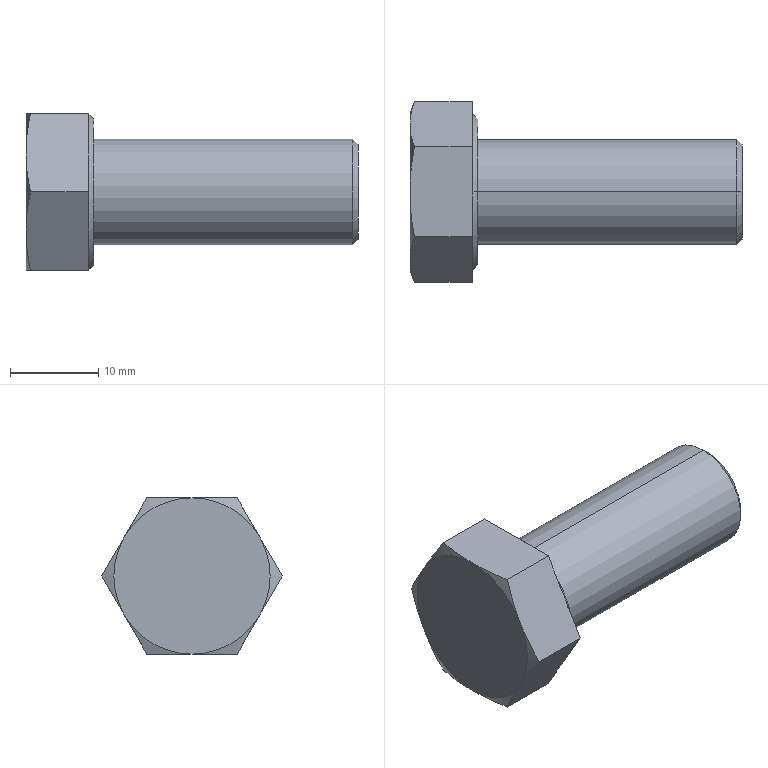Part | SolidWorks | features RevCut 3, Boss 1, Chamfer 1, Extrusion 1, Fillet 1, LPattern 1 | 1 solid | 27 faces | box 37.68 x 20.473 x 17.73 mm | volume 5450 mm3 | plane 15 | cone 10 | cylinder 2 | commonest cylinder face diameters 12 x2
STEP:
#1=CARTESIAN_POINT('',(37.68,0.,-5.4));
#2=VERTEX_POINT('',#1);
#3=CARTESIAN_POINT('',(37.68,0.,5.4));
#4=VERTEX_POINT('',#3);
#5=CARTESIAN_POINT('',(37.68,0.,0.));
#6=DIRECTION('',(1.,0.,0.));
#7=DIRECTION('',(0.,0.,-1.));
#8=AXIS2_PLACEMENT_3D('',#5,#6,#7);
#9=CIRCLE('',#8,5.4);
#10=EDGE_CURVE('',#2,#4,#9,.T.);
#11=ORIENTED_EDGE('',*,*,#10,.F.);
#12=CARTESIAN_POINT('',(37.08,0.,-6.));
#13=VERTEX_POINT('',#12);
#14=CARTESIAN_POINT('',(37.68,0.,-5.4));
#15=DIRECTION('',(-0.7071,0.,-0.7071));
#16=VECTOR('',#15,1000.);
#17=LINE('',#14,#16);
#18=EDGE_CURVE('',#2,#13,#17,.T.);
#19=ORIENTED_EDGE('',*,*,#18,.T.);
#20=CARTESIAN_POINT('',(37.08,0.,6.));
#21=VERTEX_POINT('',#20);
#22=CARTESIAN_POINT('',(37.08,0.,0.));
#23=DIRECTION('',(-1.,0.,0.));
#24=DIRECTION('',(0.,0.,-1.));
#25=AXIS2_PLACEMENT_3D('',#22,#23,#24);
#26=CIRCLE('',#25,6.);
#27=EDGE_CURVE('',#21,#13,#26,.T.);
#28=ORIENTED_EDGE('',*,*,#27,.F.);
#29=CARTESIAN_POINT('',(37.68,0.,5.4));
#30=DIRECTION('',(-0.7071,0.,0.7071));
#31=VECTOR('',#30,1000.);
#32=LINE('',#29,#31);
#33=EDGE_CURVE('',#4,#21,#32,.T.);
#34=ORIENTED_EDGE('',*,*,#33,.F.);
#35=EDGE_LOOP('',(#11,#19,#28,#34));
#36=FACE_OUTER_BOUND('',#35,.T.);
#37=CARTESIAN_POINT('',(37.68,0.,0.));
#38=DIRECTION('',(-1.,0.,0.));
#39=DIRECTION('',(0.,0.,1.));
#40=AXIS2_PLACEMENT_3D('',#37,#38,#39);
#41=CONICAL_SURFACE('',#40,5.4,0.7854);
#42=ADVANCED_FACE('',(#36),#41,.T.);
#43=ORIENTED_EDGE('',*,*,#27,.T.);
#44=CARTESIAN_POINT('',(7.68,0.,-6.));
#45=VERTEX_POINT('',#44);
#46=CARTESIAN_POINT('',(37.68,0.,-6.));
#47=DIRECTION('',(-1.,0.,0.));
#48=VECTOR('',#47,1000.);
#49=LINE('',#46,#48);
#50=EDGE_CURVE('',#13,#45,#49,.T.);
#51=ORIENTED_EDGE('',*,*,#50,.T.);
#52=CARTESIAN_POINT('',(7.68,0.,6.));
#53=VERTEX_POINT('',#52);
#54=CARTESIAN_POINT('',(7.68,0.,0.));
#55=DIRECTION('',(1.,0.,0.));
#56=DIRECTION('',(0.,0.,-1.));
#57=AXIS2_PLACEMENT_3D('',#54,#55,#56);
#58=CIRCLE('',#57,6.);
#59=EDGE_CURVE('',#45,#53,#58,.T.);
#60=ORIENTED_EDGE('',*,*,#59,.T.);
#61=CARTESIAN_POINT('',(37.68,0.,6.));
#62=DIRECTION('',(-1.,0.,0.));
#63=VECTOR('',#62,1000.);
#64=LINE('',#61,#63);
#65=EDGE_CURVE('',#21,#53,#64,.T.);
#66=ORIENTED_EDGE('',*,*,#65,.F.);
#67=EDGE_LOOP('',(#43,#51,#60,#66));
#68=FACE_OUTER_BOUND('',#67,.T.);
#69=CARTESIAN_POINT('',(37.68,0.,0.));
#70=DIRECTION('',(-1.,0.,0.));
#71=DIRECTION('',(0.,0.,1.));
#72=AXIS2_PLACEMENT_3D('',#69,#70,#71);
#73=CYLINDRICAL_SURFACE('',#72,6.);
#74=ADVANCED_FACE('',(#68),#73,.T.);
#75=CARTESIAN_POINT('',(7.68,0.,8.315));
#76=VERTEX_POINT('',#75);
#77=CARTESIAN_POINT('',(7.68,0.,-8.315));
#78=VERTEX_POINT('',#77);
#79=CARTESIAN_POINT('',(7.68,0.,0.));
#80=DIRECTION('',(-1.,0.,0.));
#81=DIRECTION('',(0.,0.,1.));
#82=AXIS2_PLACEMENT_3D('',#79,#80,#81);
#83=CIRCLE('',#82,8.315);
#84=EDGE_CURVE('',#76,#78,#83,.T.);
#85=ORIENTED_EDGE('',*,*,#84,.T.);
#86=CARTESIAN_POINT('',(7.13,0.,-8.865));
#87=VERTEX_POINT('',#86);
#88=CARTESIAN_POINT('',(7.08,0.,-8.915));
#89=DIRECTION('',(-0.7071,0.,-0.7071));
#90=VECTOR('',#89,1000.);
#91=LINE('',#88,#90);
#92=EDGE_CURVE('',#78,#87,#91,.T.);
#93=ORIENTED_EDGE('',*,*,#92,.T.);
#94=CARTESIAN_POINT('',(7.08,0.9429,-8.865));
#95=VERTEX_POINT('',#94);
#96=CARTESIAN_POINT('',(7.13,0.,-8.865));
#97=CARTESIAN_POINT('',(7.13,0.3145,-8.865));
#98=CARTESIAN_POINT('',(7.113,0.6288,-8.865));
#99=CARTESIAN_POINT('',(7.08,0.9429,-8.865));
#100=B_SPLINE_CURVE_WITH_KNOTS('',3,(#96,#97,#98,#99),.UNSPECIFIED.,.F.,.F.,(4,4),(0.004972,0.005912),.UNSPECIFIED.);
#101=EDGE_CURVE('',#87,#95,#100,.T.);
#102=ORIENTED_EDGE('',*,*,#101,.T.);
#103=CARTESIAN_POINT('',(7.08,7.206,-5.249));
#104=VERTEX_POINT('',#103);
#105=CARTESIAN_POINT('',(7.08,0.,0.));
#106=DIRECTION('',(-1.,0.,0.));
#107=DIRECTION('',(0.,0.,1.));
#108=AXIS2_PLACEMENT_3D('',#105,#106,#107);
#109=CIRCLE('',#108,8.915);
#110=EDGE_CURVE('',#104,#95,#109,.T.);
#111=ORIENTED_EDGE('',*,*,#110,.F.);
#112=CARTESIAN_POINT('',(7.08,8.149,-3.616));
#113=VERTEX_POINT('',#112);
#114=CARTESIAN_POINT('',(7.08,7.206,-5.249));
#115=CARTESIAN_POINT('',(7.146,7.52,-4.705));
#116=CARTESIAN_POINT('',(7.146,7.834,-4.16));
#117=CARTESIAN_POINT('',(7.08,8.149,-3.616));
#118=B_SPLINE_CURVE_WITH_KNOTS('',3,(#114,#115,#116,#117),.UNSPECIFIED.,.F.,.F.,(4,4),(0.000001889,0.001888),.UNSPECIFIED.);
#119=EDGE_CURVE('',#104,#113,#118,.T.);
#120=ORIENTED_EDGE('',*,*,#119,.T.);
#121=CARTESIAN_POINT('',(7.08,8.149,3.616));
#122=VERTEX_POINT('',#121);
#123=CARTESIAN_POINT('',(7.08,0.,0.));
#124=DIRECTION('',(-1.,0.,0.));
#125=DIRECTION('',(0.,0.,1.));
#126=AXIS2_PLACEMENT_3D('',#123,#124,#125);
#127=CIRCLE('',#126,8.915);
#128=EDGE_CURVE('',#122,#113,#127,.T.);
#129=ORIENTED_EDGE('',*,*,#128,.F.);
#130=CARTESIAN_POINT('',(7.08,7.206,5.249));
#131=VERTEX_POINT('',#130);
#132=CARTESIAN_POINT('',(7.08,8.149,3.616));
#133=CARTESIAN_POINT('',(7.146,7.834,4.16));
#134=CARTESIAN_POINT('',(7.146,7.52,4.705));
#135=CARTESIAN_POINT('',(7.08,7.206,5.249));
#136=B_SPLINE_CURVE_WITH_KNOTS('',3,(#132,#133,#134,#135),.UNSPECIFIED.,.F.,.F.,(4,4),(0.000001889,0.001888),.UNSPECIFIED.);
#137=EDGE_CURVE('',#122,#131,#136,.T.);
#138=ORIENTED_EDGE('',*,*,#137,.T.);
#139=CARTESIAN_POINT('',(7.08,0.9429,8.865));
#140=VERTEX_POINT('',#139);
#141=CARTESIAN_POINT('',(7.08,0.,0.));
#142=DIRECTION('',(-1.,0.,0.));
#143=DIRECTION('',(0.,0.,1.));
#144=AXIS2_PLACEMENT_3D('',#141,#142,#143);
#145=CIRCLE('',#144,8.915);
#146=EDGE_CURVE('',#140,#131,#145,.T.);
#147=ORIENTED_EDGE('',*,*,#146,.F.);
#148=CARTESIAN_POINT('',(7.13,0.,8.865));
#149=VERTEX_POINT('',#148);
#150=CARTESIAN_POINT('',(7.08,0.9429,8.865));
#151=CARTESIAN_POINT('',(7.113,0.6288,8.865));
#152=CARTESIAN_POINT('',(7.13,0.3145,8.865));
#153=CARTESIAN_POINT('',(7.13,0.,8.865));
#154=B_SPLINE_CURVE_WITH_KNOTS('',3,(#150,#151,#152,#153),.UNSPECIFIED.,.F.,.F.,(4,4),(0.004457,0.005396),.UNSPECIFIED.);
#155=EDGE_CURVE('',#140,#149,#154,.T.);
#156=ORIENTED_EDGE('',*,*,#155,.T.);
#157=CARTESIAN_POINT('',(7.08,0.,8.915));
#158=DIRECTION('',(-0.7071,0.,0.7071));
#159=VECTOR('',#158,1000.);
#160=LINE('',#157,#159);
#161=EDGE_CURVE('',#76,#149,#160,.T.);
#162=ORIENTED_EDGE('',*,*,#161,.F.);
#163=EDGE_LOOP('',(#85,#93,#102,#111,#120,#129,#138,#147,#156,#162));
#164=FACE_OUTER_BOUND('',#163,.T.);
#165=CARTESIAN_POINT('',(7.08,0.,0.));
#166=DIRECTION('',(-1.,0.,0.));
#167=DIRECTION('',(0.,0.,1.));
#168=AXIS2_PLACEMENT_3D('',#165,#166,#167);
#169=CONICAL_SURFACE('',#168,8.915,0.7854);
#170=ADVANCED_FACE('',(#164),#169,.T.);
#171=ORIENTED_EDGE('',*,*,#84,.F.);
#172=CARTESIAN_POINT('',(7.68,0.,0.));
#173=DIRECTION('',(-1.,0.,0.));
#174=DIRECTION('',(0.,0.,1.));
#175=AXIS2_PLACEMENT_3D('',#172,#173,#174);
#176=CIRCLE('',#175,8.315);
#177=EDGE_CURVE('',#78,#76,#176,.T.);
#178=ORIENTED_EDGE('',*,*,#177,.F.);
#179=EDGE_LOOP('',(#171,#178));
#180=FACE_OUTER_BOUND('',#179,.T.);
#181=CARTESIAN_POINT('',(7.68,0.,0.));
#182=DIRECTION('',(1.,0.,0.));
#183=DIRECTION('',(0.,0.,-1.));
#184=AXIS2_PLACEMENT_3D('',#181,#182,#183);
#185=CIRCLE('',#184,6.);
#186=EDGE_CURVE('',#53,#45,#185,.T.);
#187=ORIENTED_EDGE('',*,*,#186,.F.);
#188=ORIENTED_EDGE('',*,*,#59,.F.);
#189=EDGE_LOOP('',(#187,#188));
#190=FACE_BOUND('',#189,.T.);
#191=CARTESIAN_POINT('',(7.68,-5.118,-8.865));
#192=DIRECTION('',(1.,0.,0.));
#193=DIRECTION('',(0.,0.,-1.));
#194=AXIS2_PLACEMENT_3D('',#191,#192,#193);
#195=PLANE('',#194);
#196=ADVANCED_FACE('',(#180,#190),#195,.T.);
#197=CARTESIAN_POINT('',(0.4992,-5.118,-8.865));
#198=VERTEX_POINT('',#197);
#199=CARTESIAN_POINT('',(0.,-7.677,-4.432));
#200=VERTEX_POINT('',#199);
#201=CARTESIAN_POINT('',(0.4992,-5.118,-8.865));
#202=CARTESIAN_POINT('',(0.3439,-5.545,-8.126));
#203=CARTESIAN_POINT('',(0.2179,-5.971,-7.388));
#204=CARTESIAN_POINT('',(0.04564,-6.824,-5.91));
#205=CARTESIAN_POINT('',(0.,-7.251,-5.171));
#206=CARTESIAN_POINT('',(0.,-7.677,-4.432));
#207=B_SPLINE_CURVE_WITH_KNOTS('',3,(#201,#202,#203,#204,#205,#206),.UNSPECIFIED.,.F.,.F.,(4,2,4),(0.000000231,0.002559,0.005118),.UNSPECIFIED.);
#208=EDGE_CURVE('',#198,#200,#207,.T.);
#209=ORIENTED_EDGE('',*,*,#208,.F.);
#210=CARTESIAN_POINT('',(7.08,-5.118,-8.865));
#211=VERTEX_POINT('',#210);
#212=CARTESIAN_POINT('',(7.68,-5.118,-8.865));
#213=DIRECTION('',(-1.,0.,0.));
#214=VECTOR('',#213,1000.);
#215=LINE('',#212,#214);
#216=EDGE_CURVE('',#211,#198,#215,.T.);
#217=ORIENTED_EDGE('',*,*,#216,.F.);
#218=CARTESIAN_POINT('',(7.08,-7.206,-5.249));
#219=VERTEX_POINT('',#218);
#220=CARTESIAN_POINT('',(7.08,-10.236,0.));
#221=DIRECTION('',(0.,0.5,-0.866));
#222=VECTOR('',#221,1000.);
#223=LINE('',#220,#222);
#224=EDGE_CURVE('',#219,#211,#223,.T.);
#225=ORIENTED_EDGE('',*,*,#224,.F.);
#226=CARTESIAN_POINT('',(7.08,-8.149,-3.616));
#227=VERTEX_POINT('',#226);
#228=CARTESIAN_POINT('',(7.08,-8.149,-3.616));
#229=CARTESIAN_POINT('',(7.146,-7.834,-4.16));
#230=CARTESIAN_POINT('',(7.146,-7.52,-4.705));
#231=CARTESIAN_POINT('',(7.08,-7.206,-5.249));
#232=B_SPLINE_CURVE_WITH_KNOTS('',3,(#228,#229,#230,#231),.UNSPECIFIED.,.F.,.F.,(4,4),(0.000001889,0.001888),.UNSPECIFIED.);
#233=EDGE_CURVE('',#227,#219,#232,.T.);
#234=ORIENTED_EDGE('',*,*,#233,.F.);
#235=CARTESIAN_POINT('',(7.08,-10.236,0.));
#236=VERTEX_POINT('',#235);
#237=CARTESIAN_POINT('',(7.08,-10.236,0.));
#238=DIRECTION('',(0.,0.5,-0.866));
#239=VECTOR('',#238,1000.);
#240=LINE('',#237,#239);
#241=EDGE_CURVE('',#236,#227,#240,.T.);
#242=ORIENTED_EDGE('',*,*,#241,.F.);
#243=CARTESIAN_POINT('',(0.4992,-10.236,0.));
#244=VERTEX_POINT('',#243);
#245=CARTESIAN_POINT('',(7.68,-10.236,0.));
#246=DIRECTION('',(-1.,0.,0.));
#247=VECTOR('',#246,1000.);
#248=LINE('',#245,#247);
#249=EDGE_CURVE('',#236,#244,#248,.T.);
#250=ORIENTED_EDGE('',*,*,#249,.T.);
#251=CARTESIAN_POINT('',(0.,-7.677,-4.432));
#252=CARTESIAN_POINT('',(0.,-8.104,-3.694));
#253=CARTESIAN_POINT('',(0.04564,-8.53,-2.955));
#254=CARTESIAN_POINT('',(0.2179,-9.383,-1.477));
#255=CARTESIAN_POINT('',(0.3439,-9.81,-0.7387));
#256=CARTESIAN_POINT('',(0.4992,-10.236,0.));
#257=B_SPLINE_CURVE_WITH_KNOTS('',3,(#251,#252,#253,#254,#255,#256),.UNSPECIFIED.,.F.,.F.,(4,2,4),(0.005118,0.007678,0.01024),.UNSPECIFIED.);
#258=EDGE_CURVE('',#200,#244,#257,.T.);
#259=ORIENTED_EDGE('',*,*,#258,.F.);
#260=EDGE_LOOP('',(#209,#217,#225,#234,#242,#250,#259));
#261=FACE_OUTER_BOUND('',#260,.T.);
#262=CARTESIAN_POINT('',(7.68,-10.236,0.));
#263=DIRECTION('',(0.,0.866,0.5));
#264=DIRECTION('',(0.,-0.5,0.866));
#265=AXIS2_PLACEMENT_3D('',#262,#263,#264);
#266=PLANE('',#265);
#267=ADVANCED_FACE('',(#261),#266,.F.);
#268=CARTESIAN_POINT('',(0.4992,5.118,-8.865));
#269=VERTEX_POINT('',#268);
#270=CARTESIAN_POINT('',(0.,0.,-8.865));
#271=VERTEX_POINT('',#270);
#272=CARTESIAN_POINT('',(0.4992,5.118,-8.865));
#273=CARTESIAN_POINT('',(0.3443,4.267,-8.865));
#274=CARTESIAN_POINT('',(0.2182,3.415,-8.865));
#275=CARTESIAN_POINT('',(0.04582,1.709,-8.865));
#276=CARTESIAN_POINT('',(0.,0.8548,-8.865));
#277=CARTESIAN_POINT('',(0.,0.,-8.865));
#278=B_SPLINE_CURVE_WITH_KNOTS('',3,(#272,#273,#274,#275,#276,#277),.UNSPECIFIED.,.F.,.F.,(4,2,4),(0.01846,0.02104,0.02362),.UNSPECIFIED.);
#279=EDGE_CURVE('',#269,#271,#278,.T.);
#280=ORIENTED_EDGE('',*,*,#279,.F.);
#281=CARTESIAN_POINT('',(7.08,5.118,-8.865));
#282=VERTEX_POINT('',#281);
#283=CARTESIAN_POINT('',(7.68,5.118,-8.865));
#284=DIRECTION('',(-1.,0.,0.));
#285=VECTOR('',#284,1000.);
#286=LINE('',#283,#285);
#287=EDGE_CURVE('',#282,#269,#286,.T.);
#288=ORIENTED_EDGE('',*,*,#287,.F.);
#289=CARTESIAN_POINT('',(7.08,-5.118,-8.865));
#290=DIRECTION('',(0.,1.,0.));
#291=VECTOR('',#290,1000.);
#292=LINE('',#289,#291);
#293=EDGE_CURVE('',#95,#282,#292,.T.);
#294=ORIENTED_EDGE('',*,*,#293,.F.);
#295=ORIENTED_EDGE('',*,*,#101,.F.);
#296=CARTESIAN_POINT('',(7.08,-0.9429,-8.865));
#297=VERTEX_POINT('',#296);
#298=CARTESIAN_POINT('',(7.08,-0.9429,-8.865));
#299=CARTESIAN_POINT('',(7.113,-0.6284,-8.865));
#300=CARTESIAN_POINT('',(7.13,-0.3141,-8.865));
#301=CARTESIAN_POINT('',(7.13,0.,-8.865));
#302=B_SPLINE_CURVE_WITH_KNOTS('',3,(#298,#299,#300,#301),.UNSPECIFIED.,.F.,.F.,(4,4),(0.004033,0.004972),.UNSPECIFIED.);
#303=EDGE_CURVE('',#297,#87,#302,.T.);
#304=ORIENTED_EDGE('',*,*,#303,.F.);
#305=CARTESIAN_POINT('',(7.08,-5.118,-8.865));
#306=DIRECTION('',(0.,1.,0.));
#307=VECTOR('',#306,1000.);
#308=LINE('',#305,#307);
#309=EDGE_CURVE('',#211,#297,#308,.T.);
#310=ORIENTED_EDGE('',*,*,#309,.F.);
#311=ORIENTED_EDGE('',*,*,#216,.T.);
#312=CARTESIAN_POINT('',(0.,0.,-8.865));
#313=CARTESIAN_POINT('',(0.,-0.8523,-8.865));
#314=CARTESIAN_POINT('',(0.04558,-1.706,-8.865));
#315=CARTESIAN_POINT('',(0.2181,-3.414,-8.865));
#316=CARTESIAN_POINT('',(0.3449,-4.271,-8.865));
#317=CARTESIAN_POINT('',(0.4992,-5.118,-8.865));
#318=B_SPLINE_CURVE_WITH_KNOTS('',3,(#312,#313,#314,#315,#316,#317),.UNSPECIFIED.,.F.,.F.,(4,2,4),(0.02362,0.02619,0.02876),.UNSPECIFIED.);
#319=EDGE_CURVE('',#271,#198,#318,.T.);
#320=ORIENTED_EDGE('',*,*,#319,.F.);
#321=EDGE_LOOP('',(#280,#288,#294,#295,#304,#310,#311,#320));
#322=FACE_OUTER_BOUND('',#321,.T.);
#323=CARTESIAN_POINT('',(7.68,-5.118,-8.865));
#324=DIRECTION('',(0.,0.,1.));
#325=DIRECTION('',(1.,0.,0.));
#326=AXIS2_PLACEMENT_3D('',#323,#324,#325);
#327=PLANE('',#326);
#328=ADVANCED_FACE('',(#322),#327,.F.);
#329=CARTESIAN_POINT('',(0.4992,10.236,0.));
#330=VERTEX_POINT('',#329);
#331=CARTESIAN_POINT('',(0.,7.677,-4.433));
#332=VERTEX_POINT('',#331);
#333=CARTESIAN_POINT('',(0.4992,10.236,0.));
#334=CARTESIAN_POINT('',(0.3439,9.81,-0.7387));
#335=CARTESIAN_POINT('',(0.2179,9.383,-1.477));
#336=CARTESIAN_POINT('',(0.04564,8.53,-2.955));
#337=CARTESIAN_POINT('',(0.,8.104,-3.694));
#338=CARTESIAN_POINT('',(0.,7.677,-4.433));
#339=B_SPLINE_CURVE_WITH_KNOTS('',3,(#333,#334,#335,#336,#337,#338),.UNSPECIFIED.,.F.,.F.,(4,2,4),(0.000000231,0.002559,0.005118),.UNSPECIFIED.);
#340=EDGE_CURVE('',#330,#332,#339,.T.);
#341=ORIENTED_EDGE('',*,*,#340,.F.);
#342=CARTESIAN_POINT('',(7.08,10.236,0.));
#343=VERTEX_POINT('',#342);
#344=CARTESIAN_POINT('',(7.68,10.236,0.));
#345=DIRECTION('',(-1.,0.,0.));
#346=VECTOR('',#345,1000.);
#347=LINE('',#344,#346);
#348=EDGE_CURVE('',#343,#330,#347,.T.);
#349=ORIENTED_EDGE('',*,*,#348,.F.);
#350=CARTESIAN_POINT('',(7.08,5.118,-8.865));
#351=DIRECTION('',(0.,0.5,0.866));
#352=VECTOR('',#351,1000.);
#353=LINE('',#350,#352);
#354=EDGE_CURVE('',#113,#343,#353,.T.);
#355=ORIENTED_EDGE('',*,*,#354,.F.);
#356=ORIENTED_EDGE('',*,*,#119,.F.);
#357=CARTESIAN_POINT('',(7.08,5.118,-8.865));
#358=DIRECTION('',(0.,0.5,0.866));
#359=VECTOR('',#358,1000.);
#360=LINE('',#357,#359);
#361=EDGE_CURVE('',#282,#104,#360,.T.);
#362=ORIENTED_EDGE('',*,*,#361,.F.);
#363=ORIENTED_EDGE('',*,*,#287,.T.);
#364=CARTESIAN_POINT('',(0.,7.677,-4.433));
#365=CARTESIAN_POINT('',(0.,7.251,-5.171));
#366=CARTESIAN_POINT('',(0.04564,6.824,-5.91));
#367=CARTESIAN_POINT('',(0.2179,5.971,-7.387));
#368=CARTESIAN_POINT('',(0.3439,5.545,-8.126));
#369=CARTESIAN_POINT('',(0.4992,5.118,-8.865));
#370=B_SPLINE_CURVE_WITH_KNOTS('',3,(#364,#365,#366,#367,#368,#369),.UNSPECIFIED.,.F.,.F.,(4,2,4),(0.005118,0.007678,0.01024),.UNSPECIFIED.);
#371=EDGE_CURVE('',#332,#269,#370,.T.);
#372=ORIENTED_EDGE('',*,*,#371,.F.);
#373=EDGE_LOOP('',(#341,#349,#355,#356,#362,#363,#372));
#374=FACE_OUTER_BOUND('',#373,.T.);
#375=CARTESIAN_POINT('',(7.68,5.118,-8.865));
#376=DIRECTION('',(0.,-0.866,0.5));
#377=DIRECTION('',(0.,-0.5,-0.866));
#378=AXIS2_PLACEMENT_3D('',#375,#376,#377);
#379=PLANE('',#378);
#380=ADVANCED_FACE('',(#374),#379,.F.);
#381=CARTESIAN_POINT('',(0.4992,5.118,8.865));
#382=VERTEX_POINT('',#381);
#383=CARTESIAN_POINT('',(0.,7.677,4.432));
#384=VERTEX_POINT('',#383);
#385=CARTESIAN_POINT('',(0.4992,5.118,8.865));
#386=CARTESIAN_POINT('',(0.3439,5.545,8.126));
#387=CARTESIAN_POINT('',(0.2179,5.971,7.388));
#388=CARTESIAN_POINT('',(0.04564,6.824,5.91));
#389=CARTESIAN_POINT('',(0.,7.251,5.171));
#390=CARTESIAN_POINT('',(0.,7.677,4.432));
#391=B_SPLINE_CURVE_WITH_KNOTS('',3,(#385,#386,#387,#388,#389,#390),.UNSPECIFIED.,.F.,.F.,(4,2,4),(0.000000231,0.002559,0.005118),.UNSPECIFIED.);
#392=EDGE_CURVE('',#382,#384,#391,.T.);
#393=ORIENTED_EDGE('',*,*,#392,.F.);
#394=CARTESIAN_POINT('',(7.08,5.118,8.865));
#395=VERTEX_POINT('',#394);
#396=CARTESIAN_POINT('',(7.68,5.118,8.865));
#397=DIRECTION('',(-1.,0.,0.));
#398=VECTOR('',#397,1000.);
#399=LINE('',#396,#398);
#400=EDGE_CURVE('',#395,#382,#399,.T.);
#401=ORIENTED_EDGE('',*,*,#400,.F.);
#402=CARTESIAN_POINT('',(7.08,10.236,0.));
#403=DIRECTION('',(0.,-0.5,0.866));
#404=VECTOR('',#403,1000.);
#405=LINE('',#402,#404);
#406=EDGE_CURVE('',#131,#395,#405,.T.);
#407=ORIENTED_EDGE('',*,*,#406,.F.);
#408=ORIENTED_EDGE('',*,*,#137,.F.);
#409=CARTESIAN_POINT('',(7.08,10.236,0.));
#410=DIRECTION('',(0.,-0.5,0.866));
#411=VECTOR('',#410,1000.);
#412=LINE('',#409,#411);
#413=EDGE_CURVE('',#343,#122,#412,.T.);
#414=ORIENTED_EDGE('',*,*,#413,.F.);
#415=ORIENTED_EDGE('',*,*,#348,.T.);
#416=CARTESIAN_POINT('',(0.,7.677,4.432));
#417=CARTESIAN_POINT('',(0.,8.104,3.694));
#418=CARTESIAN_POINT('',(0.04564,8.53,2.955));
#419=CARTESIAN_POINT('',(0.2179,9.383,1.477));
#420=CARTESIAN_POINT('',(0.3439,9.81,0.7387));
#421=CARTESIAN_POINT('',(0.4992,10.236,0.));
#422=B_SPLINE_CURVE_WITH_KNOTS('',3,(#416,#417,#418,#419,#420,#421),.UNSPECIFIED.,.F.,.F.,(4,2,4),(0.005118,0.007678,0.01024),.UNSPECIFIED.);
#423=EDGE_CURVE('',#384,#330,#422,.T.);
#424=ORIENTED_EDGE('',*,*,#423,.F.);
#425=EDGE_LOOP('',(#393,#401,#407,#408,#414,#415,#424));
#426=FACE_OUTER_BOUND('',#425,.T.);
#427=CARTESIAN_POINT('',(7.68,10.236,0.));
#428=DIRECTION('',(0.,-0.866,-0.5));
#429=DIRECTION('',(0.,0.5,-0.866));
#430=AXIS2_PLACEMENT_3D('',#427,#428,#429);
#431=PLANE('',#430);
#432=ADVANCED_FACE('',(#426),#431,.F.);
#433=CARTESIAN_POINT('',(0.4992,-5.118,8.865));
#434=VERTEX_POINT('',#433);
#435=CARTESIAN_POINT('',(0.,0.,8.865));
#436=VERTEX_POINT('',#435);
#437=CARTESIAN_POINT('',(0.4992,-5.118,8.865));
#438=CARTESIAN_POINT('',(0.3449,-4.271,8.865));
#439=CARTESIAN_POINT('',(0.2181,-3.414,8.865));
#440=CARTESIAN_POINT('',(0.04558,-1.706,8.865));
#441=CARTESIAN_POINT('',(0.,-0.8523,8.865));
#442=CARTESIAN_POINT('',(0.,0.,8.865));
#443=B_SPLINE_CURVE_WITH_KNOTS('',3,(#437,#438,#439,#440,#441,#442),.UNSPECIFIED.,.F.,.F.,(4,2,4),(0.008707,0.01129,0.01387),.UNSPECIFIED.);
#444=EDGE_CURVE('',#434,#436,#443,.T.);
#445=ORIENTED_EDGE('',*,*,#444,.F.);
#446=CARTESIAN_POINT('',(7.08,-5.118,8.865));
#447=VERTEX_POINT('',#446);
#448=CARTESIAN_POINT('',(7.68,-5.118,8.865));
#449=DIRECTION('',(-1.,0.,0.));
#450=VECTOR('',#449,1000.);
#451=LINE('',#448,#450);
#452=EDGE_CURVE('',#447,#434,#451,.T.);
#453=ORIENTED_EDGE('',*,*,#452,.F.);
#454=CARTESIAN_POINT('',(7.08,-0.9429,8.865));
#455=VERTEX_POINT('',#454);
#456=CARTESIAN_POINT('',(7.08,5.118,8.865));
#457=DIRECTION('',(0.,-1.,0.));
#458=VECTOR('',#457,1000.);
#459=LINE('',#456,#458);
#460=EDGE_CURVE('',#455,#447,#459,.T.);
#461=ORIENTED_EDGE('',*,*,#460,.F.);
#462=CARTESIAN_POINT('',(7.13,0.,8.865));
#463=CARTESIAN_POINT('',(7.13,-0.3141,8.865));
#464=CARTESIAN_POINT('',(7.113,-0.6284,8.865));
#465=CARTESIAN_POINT('',(7.08,-0.9429,8.865));
#466=B_SPLINE_CURVE_WITH_KNOTS('',3,(#462,#463,#464,#465),.UNSPECIFIED.,.F.,.F.,(4,4),(0.005396,0.006334),.UNSPECIFIED.);
#467=EDGE_CURVE('',#149,#455,#466,.T.);
#468=ORIENTED_EDGE('',*,*,#467,.F.);
#469=ORIENTED_EDGE('',*,*,#155,.F.);
#470=CARTESIAN_POINT('',(7.08,5.118,8.865));
#471=DIRECTION('',(0.,-1.,0.));
#472=VECTOR('',#471,1000.);
#473=LINE('',#470,#472);
#474=EDGE_CURVE('',#395,#140,#473,.T.);
#475=ORIENTED_EDGE('',*,*,#474,.F.);
#476=ORIENTED_EDGE('',*,*,#400,.T.);
#477=CARTESIAN_POINT('',(0.,0.,8.865));
#478=CARTESIAN_POINT('',(0.,0.8548,8.865));
#479=CARTESIAN_POINT('',(0.04582,1.709,8.865));
#480=CARTESIAN_POINT('',(0.2182,3.415,8.865));
#481=CARTESIAN_POINT('',(0.3443,4.267,8.865));
#482=CARTESIAN_POINT('',(0.4992,5.118,8.865));
#483=B_SPLINE_CURVE_WITH_KNOTS('',3,(#477,#478,#479,#480,#481,#482),.UNSPECIFIED.,.F.,.F.,(4,2,4),(0.01387,0.01645,0.01904),.UNSPECIFIED.);
#484=EDGE_CURVE('',#436,#382,#483,.T.);
#485=ORIENTED_EDGE('',*,*,#484,.F.);
#486=EDGE_LOOP('',(#445,#453,#461,#468,#469,#475,#476,#485));
#487=FACE_OUTER_BOUND('',#486,.T.);
#488=CARTESIAN_POINT('',(7.68,5.118,8.865));
#489=DIRECTION('',(0.,0.,-1.));
#490=DIRECTION('',(-1.,0.,0.));
#491=AXIS2_PLACEMENT_3D('',#488,#489,#490);
#492=PLANE('',#491);
#493=ADVANCED_FACE('',(#487),#492,.F.);
#494=CARTESIAN_POINT('',(0.,-7.677,4.433));
#495=VERTEX_POINT('',#494);
#496=CARTESIAN_POINT('',(0.4992,-10.236,0.));
#497=CARTESIAN_POINT('',(0.3439,-9.81,0.7388));
#498=CARTESIAN_POINT('',(0.2179,-9.383,1.478));
#499=CARTESIAN_POINT('',(0.04564,-8.53,2.955));
#500=CARTESIAN_POINT('',(0.,-8.104,3.694));
#501=CARTESIAN_POINT('',(0.,-7.677,4.433));
#502=B_SPLINE_CURVE_WITH_KNOTS('',3,(#496,#497,#498,#499,#500,#501),.UNSPECIFIED.,.F.,.F.,(4,2,4),(0.000000231,0.002559,0.005118),.UNSPECIFIED.);
#503=EDGE_CURVE('',#244,#495,#502,.T.);
#504=ORIENTED_EDGE('',*,*,#503,.F.);
#505=ORIENTED_EDGE('',*,*,#249,.F.);
#506=CARTESIAN_POINT('',(7.08,-8.149,3.616));
#507=VERTEX_POINT('',#506);
#508=CARTESIAN_POINT('',(7.08,-5.118,8.865));
#509=DIRECTION('',(0.,-0.5,-0.866));
#510=VECTOR('',#509,1000.);
#511=LINE('',#508,#510);
#512=EDGE_CURVE('',#507,#236,#511,.T.);
#513=ORIENTED_EDGE('',*,*,#512,.F.);
#514=CARTESIAN_POINT('',(7.08,-7.206,5.249));
#515=VERTEX_POINT('',#514);
#516=CARTESIAN_POINT('',(7.08,-7.206,5.249));
#517=CARTESIAN_POINT('',(7.146,-7.52,4.705));
#518=CARTESIAN_POINT('',(7.146,-7.834,4.16));
#519=CARTESIAN_POINT('',(7.08,-8.149,3.616));
#520=B_SPLINE_CURVE_WITH_KNOTS('',3,(#516,#517,#518,#519),.UNSPECIFIED.,.F.,.F.,(4,4),(0.000001889,0.001888),.UNSPECIFIED.);
#521=EDGE_CURVE('',#515,#507,#520,.T.);
#522=ORIENTED_EDGE('',*,*,#521,.F.);
#523=CARTESIAN_POINT('',(7.08,-5.118,8.865));
#524=DIRECTION('',(0.,-0.5,-0.866));
#525=VECTOR('',#524,1000.);
#526=LINE('',#523,#525);
#527=EDGE_CURVE('',#447,#515,#526,.T.);
#528=ORIENTED_EDGE('',*,*,#527,.F.);
#529=ORIENTED_EDGE('',*,*,#452,.T.);
#530=CARTESIAN_POINT('',(0.,-7.677,4.433));
#531=CARTESIAN_POINT('',(0.,-7.251,5.171));
#532=CARTESIAN_POINT('',(0.04564,-6.824,5.91));
#533=CARTESIAN_POINT('',(0.2179,-5.971,7.387));
#534=CARTESIAN_POINT('',(0.3439,-5.545,8.126));
#535=CARTESIAN_POINT('',(0.4992,-5.118,8.865));
#536=B_SPLINE_CURVE_WITH_KNOTS('',3,(#530,#531,#532,#533,#534,#535),.UNSPECIFIED.,.F.,.F.,(4,2,4),(0.005118,0.007678,0.01024),.UNSPECIFIED.);
#537=EDGE_CURVE('',#495,#434,#536,.T.);
#538=ORIENTED_EDGE('',*,*,#537,.F.);
#539=EDGE_LOOP('',(#504,#505,#513,#522,#528,#529,#538));
#540=FACE_OUTER_BOUND('',#539,.T.);
#541=CARTESIAN_POINT('',(7.68,-5.118,8.865));
#542=DIRECTION('',(0.,0.866,-0.5));
#543=DIRECTION('',(0.,0.5,0.866));
#544=AXIS2_PLACEMENT_3D('',#541,#542,#543);
#545=PLANE('',#544);
#546=ADVANCED_FACE('',(#540),#545,.F.);
#547=ORIENTED_EDGE('',*,*,#224,.T.);
#548=ORIENTED_EDGE('',*,*,#309,.T.);
#549=CARTESIAN_POINT('',(7.08,0.,0.));
#550=DIRECTION('',(-1.,0.,0.));
#551=DIRECTION('',(0.,0.,1.));
#552=AXIS2_PLACEMENT_3D('',#549,#550,#551);
#553=CIRCLE('',#552,8.915);
#554=EDGE_CURVE('',#297,#219,#553,.T.);
#555=ORIENTED_EDGE('',*,*,#554,.T.);
#556=EDGE_LOOP('',(#547,#548,#555));
#557=FACE_OUTER_BOUND('',#556,.T.);
#558=CARTESIAN_POINT('',(7.08,8.915,0.));
#559=DIRECTION('',(1.,0.,0.));
#560=DIRECTION('',(0.,0.,-1.));
#561=AXIS2_PLACEMENT_3D('',#558,#559,#560);
#562=PLANE('',#561);
#563=ADVANCED_FACE('',(#557),#562,.T.);
#564=ORIENTED_EDGE('',*,*,#293,.T.);
#565=ORIENTED_EDGE('',*,*,#361,.T.);
#566=ORIENTED_EDGE('',*,*,#110,.T.);
#567=EDGE_LOOP('',(#564,#565,#566));
#568=FACE_OUTER_BOUND('',#567,.T.);
#569=CARTESIAN_POINT('',(7.08,8.915,0.));
#570=DIRECTION('',(1.,0.,0.));
#571=DIRECTION('',(0.,0.,-1.));
#572=AXIS2_PLACEMENT_3D('',#569,#570,#571);
#573=PLANE('',#572);
#574=ADVANCED_FACE('',(#568),#573,.T.);
#575=ORIENTED_EDGE('',*,*,#354,.T.);
#576=ORIENTED_EDGE('',*,*,#413,.T.);
#577=ORIENTED_EDGE('',*,*,#128,.T.);
#578=EDGE_LOOP('',(#575,#576,#577));
#579=FACE_OUTER_BOUND('',#578,.T.);
#580=CARTESIAN_POINT('',(7.08,8.915,0.));
#581=DIRECTION('',(1.,0.,0.));
#582=DIRECTION('',(0.,0.,-1.));
#583=AXIS2_PLACEMENT_3D('',#580,#581,#582);
#584=PLANE('',#583);
#585=ADVANCED_FACE('',(#579),#584,.T.);
#586=ORIENTED_EDGE('',*,*,#406,.T.);
#587=ORIENTED_EDGE('',*,*,#474,.T.);
#588=ORIENTED_EDGE('',*,*,#146,.T.);
#589=EDGE_LOOP('',(#586,#587,#588));
#590=FACE_OUTER_BOUND('',#589,.T.);
#591=CARTESIAN_POINT('',(7.08,8.915,0.));
#592=DIRECTION('',(1.,0.,0.));
#593=DIRECTION('',(0.,0.,-1.));
#594=AXIS2_PLACEMENT_3D('',#591,#592,#593);
#595=PLANE('',#594);
#596=ADVANCED_FACE('',(#590),#595,.T.);
#597=ORIENTED_EDGE('',*,*,#460,.T.);
#598=ORIENTED_EDGE('',*,*,#527,.T.);
#599=CARTESIAN_POINT('',(7.08,0.,0.));
#600=DIRECTION('',(-1.,0.,0.));
#601=DIRECTION('',(0.,0.,1.));
#602=AXIS2_PLACEMENT_3D('',#599,#600,#601);
#603=CIRCLE('',#602,8.915);
#604=EDGE_CURVE('',#515,#455,#603,.T.);
#605=ORIENTED_EDGE('',*,*,#604,.T.);
#606=EDGE_LOOP('',(#597,#598,#605));
#607=FACE_OUTER_BOUND('',#606,.T.);
#608=CARTESIAN_POINT('',(7.08,8.915,0.));
#609=DIRECTION('',(1.,0.,0.));
#610=DIRECTION('',(0.,0.,-1.));
#611=AXIS2_PLACEMENT_3D('',#608,#609,#610);
#612=PLANE('',#611);
#613=ADVANCED_FACE('',(#607),#612,.T.);
#614=ORIENTED_EDGE('',*,*,#241,.T.);
#615=CARTESIAN_POINT('',(7.08,0.,0.));
#616=DIRECTION('',(-1.,0.,0.));
#617=DIRECTION('',(0.,0.,1.));
#618=AXIS2_PLACEMENT_3D('',#615,#616,#617);
#619=CIRCLE('',#618,8.915);
#620=EDGE_CURVE('',#227,#507,#619,.T.);
#621=ORIENTED_EDGE('',*,*,#620,.T.);
#622=ORIENTED_EDGE('',*,*,#512,.T.);
#623=EDGE_LOOP('',(#614,#621,#622));
#624=FACE_OUTER_BOUND('',#623,.T.);
#625=CARTESIAN_POINT('',(7.08,8.915,0.));
#626=DIRECTION('',(1.,0.,0.));
#627=DIRECTION('',(0.,0.,-1.));
#628=AXIS2_PLACEMENT_3D('',#625,#626,#627);
#629=PLANE('',#628);
#630=ADVANCED_FACE('',(#624),#629,.T.);
#631=ORIENTED_EDGE('',*,*,#92,.F.);
#632=ORIENTED_EDGE('',*,*,#177,.T.);
#633=ORIENTED_EDGE('',*,*,#161,.T.);
#634=ORIENTED_EDGE('',*,*,#467,.T.);
#635=ORIENTED_EDGE('',*,*,#604,.F.);
#636=ORIENTED_EDGE('',*,*,#521,.T.);
#637=ORIENTED_EDGE('',*,*,#620,.F.);
#638=ORIENTED_EDGE('',*,*,#233,.T.);
#639=ORIENTED_EDGE('',*,*,#554,.F.);
#640=ORIENTED_EDGE('',*,*,#303,.T.);
#641=EDGE_LOOP('',(#631,#632,#633,#634,#635,#636,#637,#638,#639,#640));
#642=FACE_OUTER_BOUND('',#641,.T.);
#643=CARTESIAN_POINT('',(7.08,0.,0.));
#644=DIRECTION('',(-1.,0.,0.));
#645=DIRECTION('',(0.,0.,1.));
#646=AXIS2_PLACEMENT_3D('',#643,#644,#645);
#647=CONICAL_SURFACE('',#646,8.915,0.7854);
#648=ADVANCED_FACE('',(#642),#647,.T.);
#649=ORIENTED_EDGE('',*,*,#319,.T.);
#650=ORIENTED_EDGE('',*,*,#208,.T.);
#651=CARTESIAN_POINT('',(0.,0.,0.));
#652=DIRECTION('',(1.,0.,0.));
#653=DIRECTION('',(0.,0.,-1.));
#654=AXIS2_PLACEMENT_3D('',#651,#652,#653);
#655=CIRCLE('',#654,8.865);
#656=EDGE_CURVE('',#200,#271,#655,.T.);
#657=ORIENTED_EDGE('',*,*,#656,.T.);
#658=EDGE_LOOP('',(#649,#650,#657));
#659=FACE_OUTER_BOUND('',#658,.T.);
#660=CARTESIAN_POINT('',(0.,0.,0.));
#661=DIRECTION('',(1.,0.,0.));
#662=DIRECTION('',(0.,0.,-1.));
#663=AXIS2_PLACEMENT_3D('',#660,#661,#662);
#664=CONICAL_SURFACE('',#663,8.865,1.222);
#665=ADVANCED_FACE('',(#659),#664,.T.);
#666=ORIENTED_EDGE('',*,*,#258,.T.);
#667=ORIENTED_EDGE('',*,*,#503,.T.);
#668=CARTESIAN_POINT('',(0.,0.,0.));
#669=DIRECTION('',(1.,0.,0.));
#670=DIRECTION('',(0.,0.,-1.));
#671=AXIS2_PLACEMENT_3D('',#668,#669,#670);
#672=CIRCLE('',#671,8.865);
#673=EDGE_CURVE('',#495,#200,#672,.T.);
#674=ORIENTED_EDGE('',*,*,#673,.T.);
#675=EDGE_LOOP('',(#666,#667,#674));
#676=FACE_OUTER_BOUND('',#675,.T.);
#677=CARTESIAN_POINT('',(0.,0.,0.));
#678=DIRECTION('',(1.,0.,0.));
#679=DIRECTION('',(0.,0.,-1.));
#680=AXIS2_PLACEMENT_3D('',#677,#678,#679);
#681=CONICAL_SURFACE('',#680,8.865,1.222);
#682=ADVANCED_FACE('',(#676),#681,.T.);
#683=ORIENTED_EDGE('',*,*,#444,.T.);
#684=CARTESIAN_POINT('',(0.,0.,0.));
#685=DIRECTION('',(1.,0.,0.));
#686=DIRECTION('',(0.,0.,-1.));
#687=AXIS2_PLACEMENT_3D('',#684,#685,#686);
#688=CIRCLE('',#687,8.865);
#689=EDGE_CURVE('',#436,#495,#688,.T.);
#690=ORIENTED_EDGE('',*,*,#689,.T.);
#691=ORIENTED_EDGE('',*,*,#537,.T.);
#692=EDGE_LOOP('',(#683,#690,#691));
#693=FACE_OUTER_BOUND('',#692,.T.);
#694=CARTESIAN_POINT('',(0.,0.,0.));
#695=DIRECTION('',(1.,0.,0.));
#696=DIRECTION('',(0.,0.,-1.));
#697=AXIS2_PLACEMENT_3D('',#694,#695,#696);
#698=CONICAL_SURFACE('',#697,8.865,1.222);
#699=ADVANCED_FACE('',(#693),#698,.T.);
#700=ORIENTED_EDGE('',*,*,#392,.T.);
#701=CARTESIAN_POINT('',(0.,0.,0.));
#702=DIRECTION('',(-1.,0.,0.));
#703=DIRECTION('',(0.,0.,1.));
#704=AXIS2_PLACEMENT_3D('',#701,#702,#703);
#705=CIRCLE('',#704,8.865);
#706=EDGE_CURVE('',#436,#384,#705,.T.);
#707=ORIENTED_EDGE('',*,*,#706,.F.);
#708=ORIENTED_EDGE('',*,*,#484,.T.);
#709=EDGE_LOOP('',(#700,#707,#708));
#710=FACE_OUTER_BOUND('',#709,.T.);
#711=CARTESIAN_POINT('',(0.,0.,0.));
#712=DIRECTION('',(1.,0.,0.));
#713=DIRECTION('',(0.,0.,-1.));
#714=AXIS2_PLACEMENT_3D('',#711,#712,#713);
#715=CONICAL_SURFACE('',#714,8.865,1.222);
#716=ADVANCED_FACE('',(#710),#715,.T.);
#717=ORIENTED_EDGE('',*,*,#340,.T.);
#718=CARTESIAN_POINT('',(0.,0.,0.));
#719=DIRECTION('',(1.,0.,0.));
#720=DIRECTION('',(0.,0.,-1.));
#721=AXIS2_PLACEMENT_3D('',#718,#719,#720);
#722=CIRCLE('',#721,8.865);
#723=EDGE_CURVE('',#332,#384,#722,.T.);
#724=ORIENTED_EDGE('',*,*,#723,.T.);
#725=ORIENTED_EDGE('',*,*,#423,.T.);
#726=EDGE_LOOP('',(#717,#724,#725));
#727=FACE_OUTER_BOUND('',#726,.T.);
#728=CARTESIAN_POINT('',(0.,0.,0.));
#729=DIRECTION('',(1.,0.,0.));
#730=DIRECTION('',(0.,0.,-1.));
#731=AXIS2_PLACEMENT_3D('',#728,#729,#730);
#732=CONICAL_SURFACE('',#731,8.865,1.222);
#733=ADVANCED_FACE('',(#727),#732,.T.);
#734=ORIENTED_EDGE('',*,*,#371,.T.);
#735=ORIENTED_EDGE('',*,*,#279,.T.);
#736=CARTESIAN_POINT('',(0.,0.,0.));
#737=DIRECTION('',(1.,0.,0.));
#738=DIRECTION('',(0.,0.,-1.));
#739=AXIS2_PLACEMENT_3D('',#736,#737,#738);
#740=CIRCLE('',#739,8.865);
#741=EDGE_CURVE('',#271,#332,#740,.T.);
#742=ORIENTED_EDGE('',*,*,#741,.T.);
#743=EDGE_LOOP('',(#734,#735,#742));
#744=FACE_OUTER_BOUND('',#743,.T.);
#745=CARTESIAN_POINT('',(0.,0.,0.));
#746=DIRECTION('',(1.,0.,0.));
#747=DIRECTION('',(0.,0.,-1.));
#748=AXIS2_PLACEMENT_3D('',#745,#746,#747);
#749=CONICAL_SURFACE('',#748,8.865,1.222);
#750=ADVANCED_FACE('',(#744),#749,.T.);
#751=ORIENTED_EDGE('',*,*,#741,.F.);
#752=ORIENTED_EDGE('',*,*,#656,.F.);
#753=ORIENTED_EDGE('',*,*,#673,.F.);
#754=ORIENTED_EDGE('',*,*,#689,.F.);
#755=ORIENTED_EDGE('',*,*,#706,.T.);
#756=ORIENTED_EDGE('',*,*,#723,.F.);
#757=EDGE_LOOP('',(#751,#752,#753,#754,#755,#756));
#758=FACE_OUTER_BOUND('',#757,.T.);
#759=CARTESIAN_POINT('',(0.,-5.118,-8.865));
#760=DIRECTION('',(1.,0.,0.));
#761=DIRECTION('',(0.,0.,-1.));
#762=AXIS2_PLACEMENT_3D('',#759,#760,#761);
#763=PLANE('',#762);
#764=ADVANCED_FACE('',(#758),#763,.F.);
#765=ORIENTED_EDGE('',*,*,#50,.F.);
#766=CARTESIAN_POINT('',(37.08,0.,0.));
#767=DIRECTION('',(-1.,0.,0.));
#768=DIRECTION('',(0.,0.,-1.));
#769=AXIS2_PLACEMENT_3D('',#766,#767,#768);
#770=CIRCLE('',#769,6.);
#771=EDGE_CURVE('',#13,#21,#770,.T.);
#772=ORIENTED_EDGE('',*,*,#771,.T.);
#773=ORIENTED_EDGE('',*,*,#65,.T.);
#774=ORIENTED_EDGE('',*,*,#186,.T.);
#775=EDGE_LOOP('',(#765,#772,#773,#774));
#776=FACE_OUTER_BOUND('',#775,.T.);
#777=CARTESIAN_POINT('',(37.68,0.,0.));
#778=DIRECTION('',(-1.,0.,0.));
#779=DIRECTION('',(0.,0.,1.));
#780=AXIS2_PLACEMENT_3D('',#777,#778,#779);
#781=CYLINDRICAL_SURFACE('',#780,6.);
#782=ADVANCED_FACE('',(#776),#781,.T.);
#783=CARTESIAN_POINT('',(37.68,0.,0.));
#784=DIRECTION('',(1.,0.,0.));
#785=DIRECTION('',(0.,0.,-1.));
#786=AXIS2_PLACEMENT_3D('',#783,#784,#785);
#787=CIRCLE('',#786,5.4);
#788=EDGE_CURVE('',#4,#2,#787,.T.);
#789=ORIENTED_EDGE('',*,*,#788,.T.);
#790=ORIENTED_EDGE('',*,*,#10,.T.);
#791=EDGE_LOOP('',(#789,#790));
#792=FACE_OUTER_BOUND('',#791,.T.);
#793=CARTESIAN_POINT('',(37.68,0.,0.));
#794=DIRECTION('',(1.,0.,0.));
#795=DIRECTION('',(0.,0.,-1.));
#796=AXIS2_PLACEMENT_3D('',#793,#794,#795);
#797=PLANE('',#796);
#798=ADVANCED_FACE('',(#792),#797,.T.);
#799=ORIENTED_EDGE('',*,*,#18,.F.);
#800=ORIENTED_EDGE('',*,*,#788,.F.);
#801=ORIENTED_EDGE('',*,*,#33,.T.);
#802=ORIENTED_EDGE('',*,*,#771,.F.);
#803=EDGE_LOOP('',(#799,#800,#801,#802));
#804=FACE_OUTER_BOUND('',#803,.T.);
#805=CARTESIAN_POINT('',(37.68,0.,0.));
#806=DIRECTION('',(-1.,0.,0.));
#807=DIRECTION('',(0.,0.,1.));
#808=AXIS2_PLACEMENT_3D('',#805,#806,#807);
#809=CONICAL_SURFACE('',#808,5.4,0.7854);
#810=ADVANCED_FACE('',(#804),#809,.T.);
#811=CLOSED_SHELL('',(#42,#74,#170,#196,#267,#328,#380,#432,#493,#546,#563,#574,#585,#596,#613,#630,#648,#665,#682,#699,#716,#733,#750,#764,#782,#798,#810));
#812=MANIFOLD_SOLID_BREP('',#811);
#813=CARTESIAN_POINT('',(0.,0.,0.));
#814=DIRECTION('',(0.,0.,1.));
#815=DIRECTION('',(1.,0.,0.));
#816=AXIS2_PLACEMENT_3D('',#813,#814,#815);
#817=(LENGTH_UNIT()NAMED_UNIT(*)SI_UNIT(.MILLI.,.METRE.));
#818=UNCERTAINTY_MEASURE_WITH_UNIT(LENGTH_MEASURE(0.00001),#817,'','');
#819=(NAMED_UNIT(*)PLANE_ANGLE_UNIT()SI_UNIT($,.RADIAN.));
#820=(NAMED_UNIT(*)SI_UNIT($,.STERADIAN.)SOLID_ANGLE_UNIT());
#821=(GEOMETRIC_REPRESENTATION_CONTEXT(3)GLOBAL_UNCERTAINTY_ASSIGNED_CONTEXT((#818))GLOBAL_UNIT_ASSIGNED_CONTEXT((#817,#819,#820))REPRESENTATION_CONTEXT('',''));
#822=ADVANCED_BREP_SHAPE_REPRESENTATION('',(#812,#816),#821);